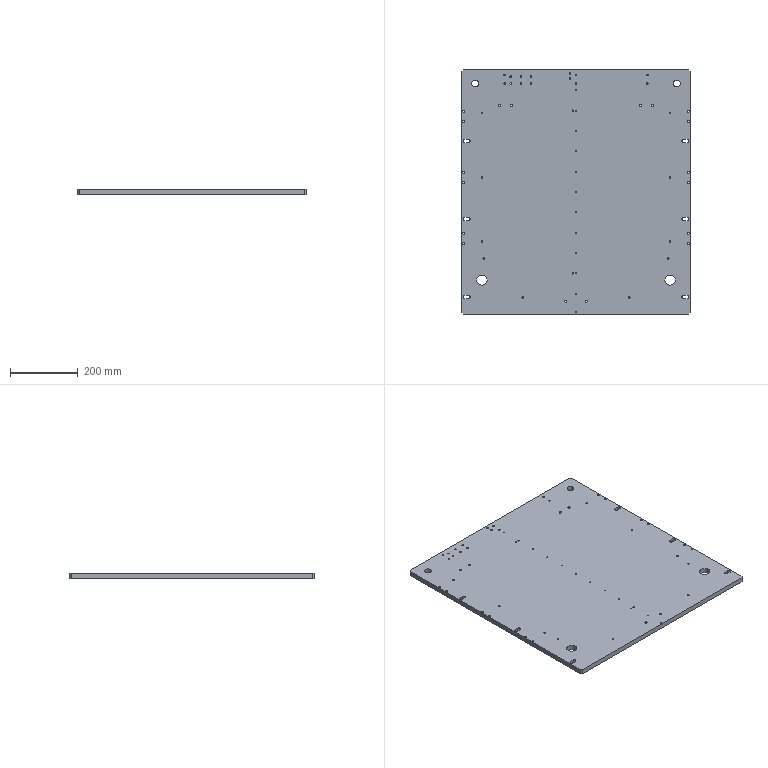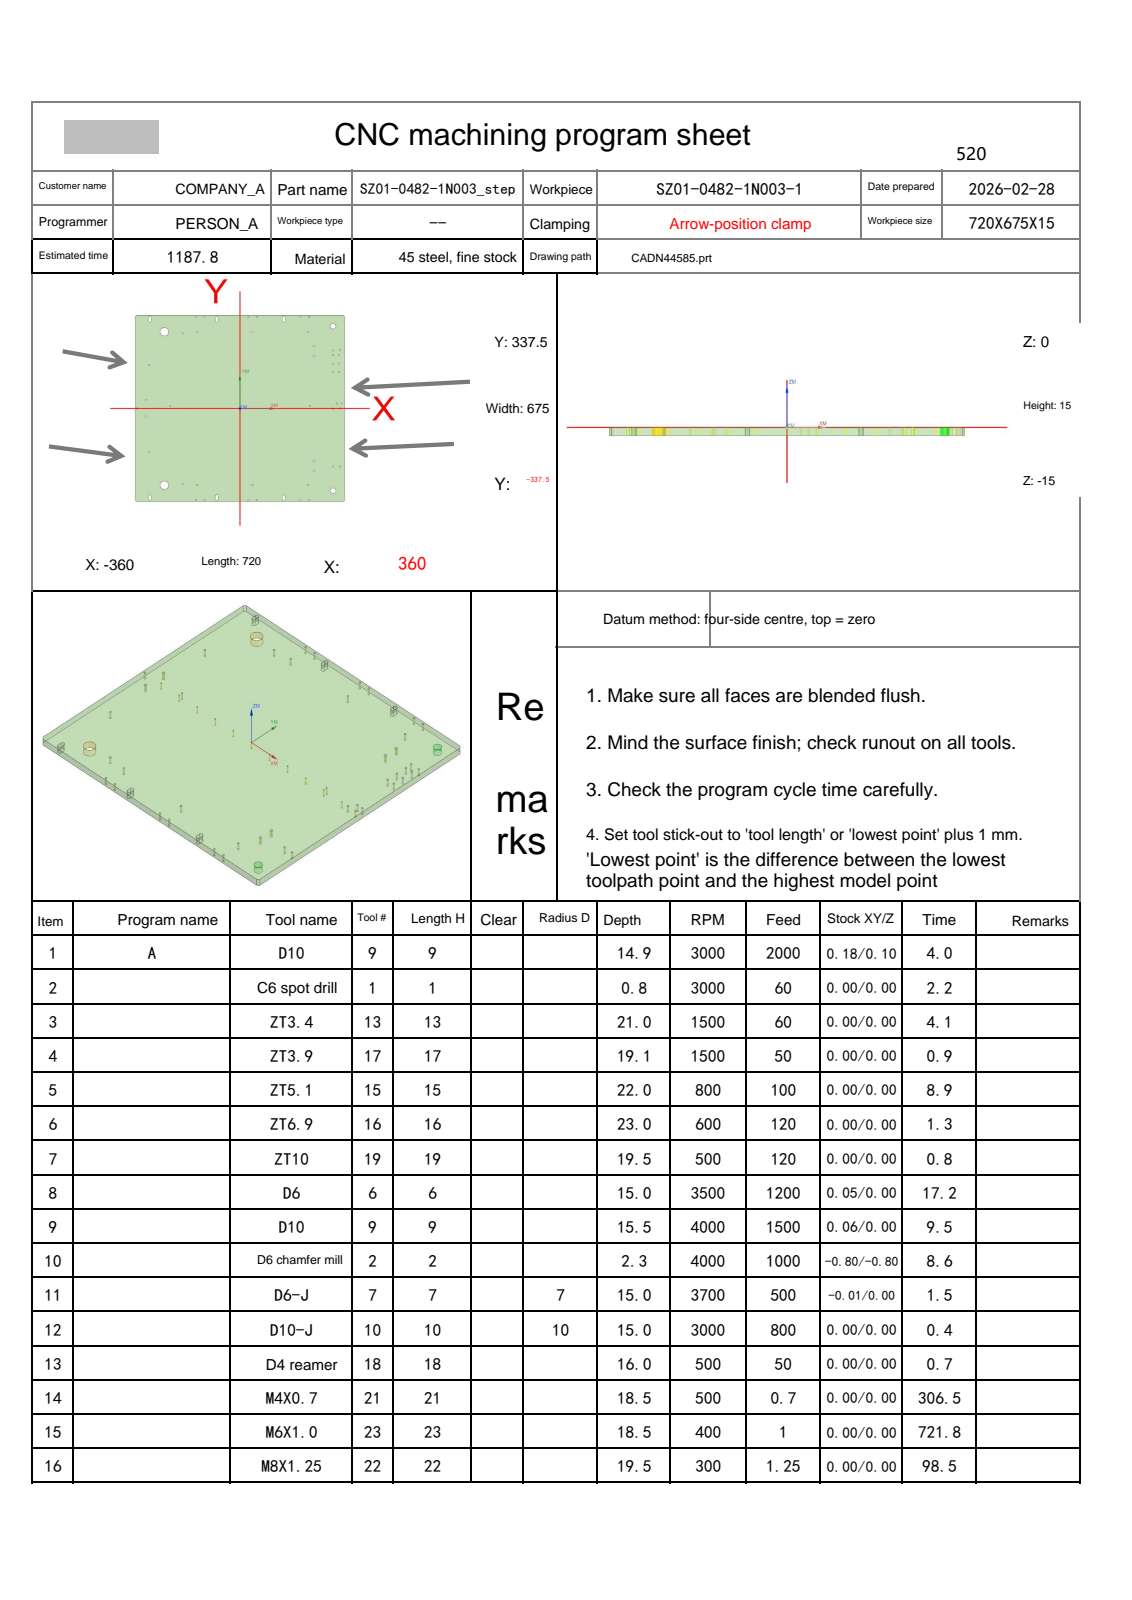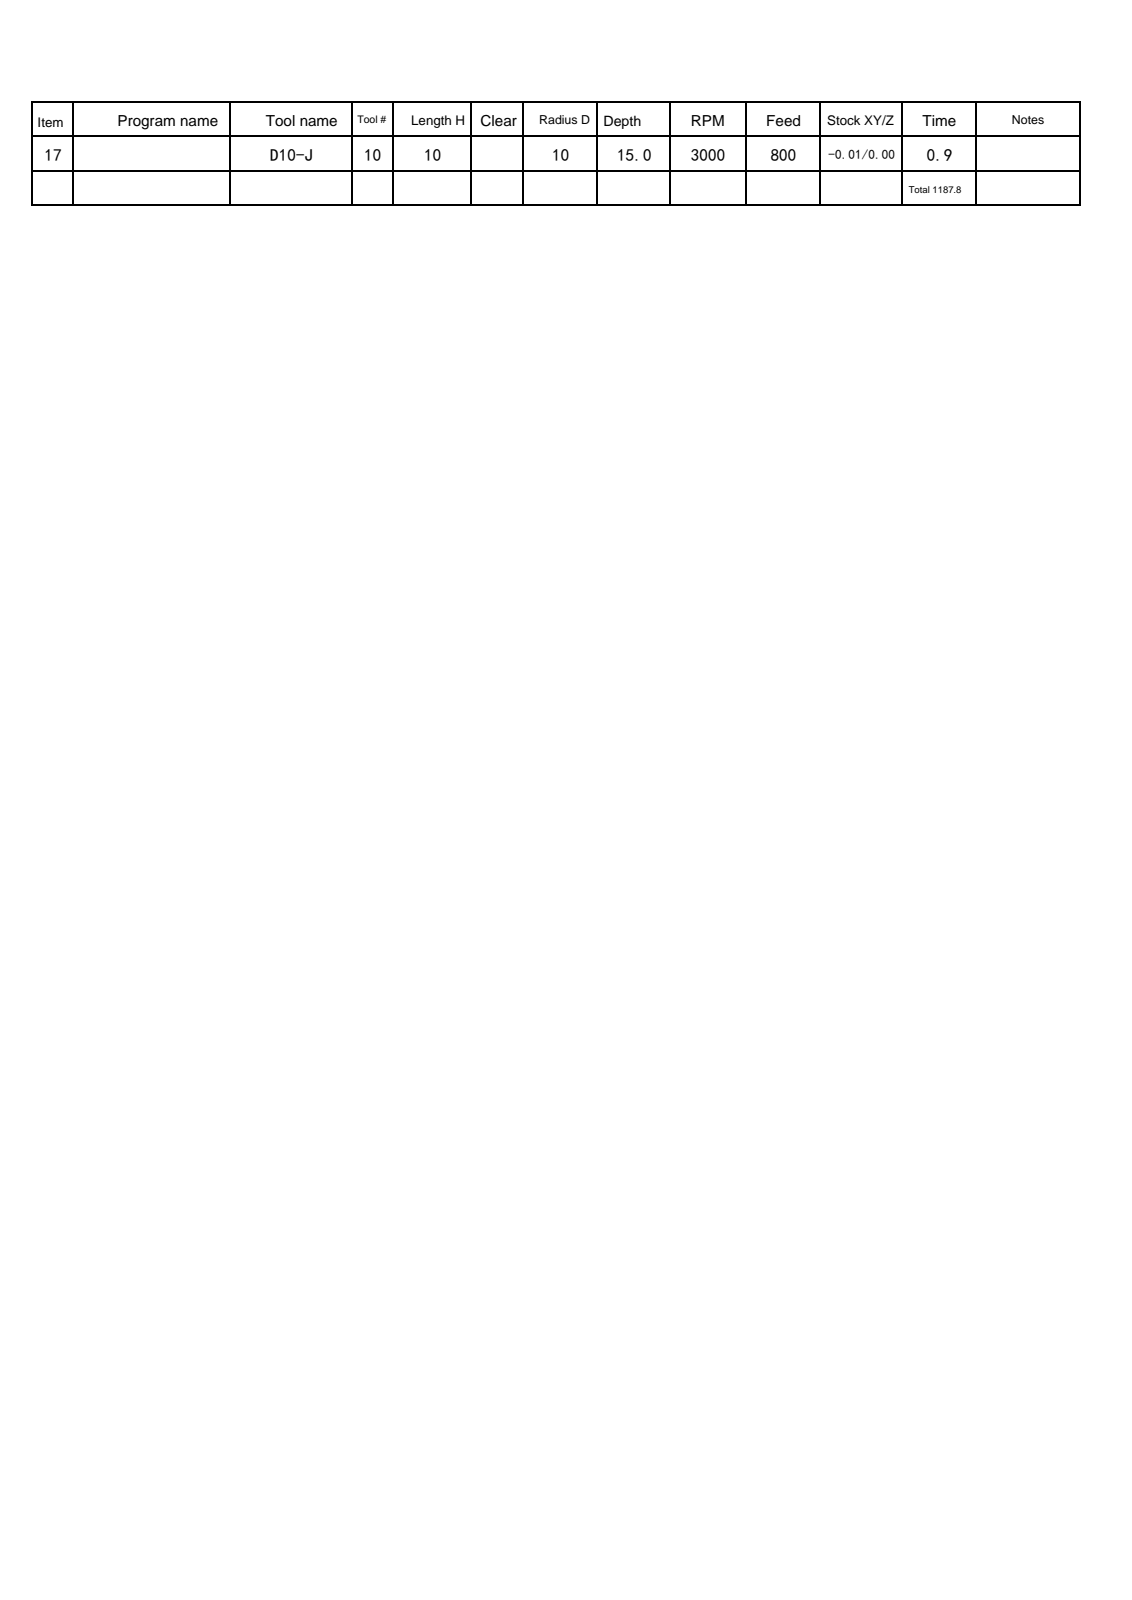NC program | NX | posted by the shop | part box 675 x 720 x 15 mm
Lines 7671 to 7907 of 7907:
N14 T21 M06
(M4X0.7 D=3.3 DR_a=180 H=21)
G00 G90 G54 X-300. Y0.0 M03 S500
G43 H21 Z30.
M08
G95
G98 G84 X-300. Y0.0 Z-18.5 R1. F.7 Q1.
X-240.
X-180.
X-120.
X-60.
X0.0
X60.
X120.
X180.
X240.
X300.
G80
G94
G00 Z30.
G91 G28 Z0.0
M05
M09
G91 G28 Z0.0
M01
N15 T23 M06
(M6X1.0 D=5. DR_a=180 H=23)
G00 G90 G54 X320. Y0.0 M03 S400
G43 H23 Z30.
M08
G95
G98 G84 X320. Y0.0 Z-18.5 R1. F1. Q2.
X345.
X350. Y18.
X334.
X340. Y132.5
X320.
Y162.5
X340.
Y192.5
X345. Y210.
X320. Y192.5
Y210.
X233. Y277.
X238. Y331.5
X208.
X58.
X28.
X43. Y277.
X-122. Y331.5
X-152.
X-147. Y277.
X-197. Y271.932
X-311.932 Y157.
X-354. Y0.0
X-311.932 Y-157.
X-197. Y-271.932
X-147. Y-277.
X-152. Y-331.5
X-122.
X43. Y-277.
X28. Y-331.5
X58.
X208.
X238.
X233. Y-277.
X320. Y-210.
X345.
G80
G94
G00 Z30.
G91 G28 Z0.0
M05
M09
G91 G28 Z0.0
M01
N16 T22 M06
(M8X1.25 D=6.8 DR_a=180 H=22)
G00 G90 G54 X255. Y225.5 M03 S300
G43 H22 Z30.
M08
G95
G98 G84 X255. Y225.5 Z-19.5 R1. F1.25 Q3.
Y189.5
Y-189.5
Y-225.5
X-322. Y-30.
Y30.
G80
G94
G00 Z30.
G91 G28 Z0.0
M05
M09
G91 G28 Z0.0
M01
N17 T10 M06
(D10-J  D=10. R=0. H=10 ce=-0.01 di=0.00)
G00 G90 G54 X322.973 Y296. M03 S3000
G43 H10 Z10.
M08
Z-6.
G01 Z-7.5 F600.
G41 D10
X323.51
G03 X325.01 Y297.5 I0.0 J1.5
X320. Y302.51 I-5.01 J0.0
X314.99 Y297.5 I0.0 J-5.01
X320. Y292.49 I5.01 J0.0
X325.01 Y297.5 I0.0 J5.01
X324.994 Y297.9 I-5.01 J0.0
X323.499 Y299.28 I-1.495 J-.12
G01 X323.379 Y299.275
X323.044 Y299.248
G40 X322.844 Y299.232
Z-6.
G00 X322.973 Y296.
Z-13.5
G01 Z-15.
G41 D10
X323.51
G03 X325.01 Y297.5 I0.0 J1.5
X320. Y302.51 I-5.01 J0.0
X314.99 Y297.5 I0.0 J-5.01
X320. Y292.49 I5.01 J0.0
X325.01 Y297.5 I0.0 J5.01
X324.994 Y297.9 I-5.01 J0.0
X323.499 Y299.28 I-1.495 J-.12
G01 X323.379 Y299.275
X323.044 Y299.248
G40 X322.844 Y299.232
Z-13.5
G00 Z10.
X322.973 Y-299.
Z-6.
G01 Z-7.5
G41 D10
X323.51
G03 X325.01 Y-297.5 I0.0 J1.5
X320. Y-292.49 I-5.01 J0.0
X314.99 Y-297.5 I0.0 J-5.01
X320. Y-302.51 I5.01 J0.0
X325.01 Y-297.5 I0.0 J5.01
X324.994 Y-297.1 I-5.01 J0.0
X323.499 Y-295.72 I-1.495 J-.12
G01 X323.379 Y-295.725
X323.044 Y-295.752
G40 X322.844 Y-295.768
Z-6.
G00 X322.973 Y-299.
Z-13.5
G01 Z-15.
G41 D10
X323.51
G03 X325.01 Y-297.5 I0.0 J1.5
X320. Y-292.49 I-5.01 J0.0
X314.99 Y-297.5 I0.0 J-5.01
X320. Y-302.51 I5.01 J0.0
X325.01 Y-297.5 I0.0 J5.01
X324.994 Y-297.1 I-5.01 J0.0
X323.499 Y-295.72 I-1.495 J-.12
G01 X323.379 Y-295.725
X323.044 Y-295.752
G40 X322.844 Y-295.768
Z-13.5
G00 Z10.
G00 G90 X354.293 Y345.278 M03 S3000
Z60.
Z-7.
G01 Z-8. F800.
X358.536 Y341.036
X363.536 Y336.036
X367.778 Y331.793
Z-7.
G00 Z60.
X354.293 Y345.278
Z-14.
G01 Z-15.
X358.536 Y341.036
X363.536 Y336.036
X367.778 Y331.793
Z-14.
G00 Z60.
Y-331.793
Z-7.
G01 Z-8.
X363.536 Y-336.036
X358.536 Y-341.036
X354.293 Y-345.278
Z-7.
G00 Z60.
X367.778 Y-331.793
Z-14.
G01 Z-15.
X363.536 Y-336.036
X358.536 Y-341.036
X354.293 Y-345.278
Z-14.
G00 Z60.
X-354.293
Z-7.
G01 Z-8.
X-358.536 Y-341.036
X-363.536 Y-336.036
X-367.778 Y-331.793
Z-7.
G00 Z60.
X-354.293 Y-345.278
Z-14.
G01 Z-15.
X-358.536 Y-341.036
X-363.536 Y-336.036
X-367.778 Y-331.793
Z-14.
G00 Z60.
Y331.793
Z-7.
G01 Z-8.
X-363.536 Y336.036
X-358.536 Y341.036
X-354.293 Y345.278
Z-7.
G00 Z60.
X-367.778 Y331.793
Z-14.
G01 Z-15.
X-363.536 Y336.036
X-358.536 Y341.036
X-354.293 Y345.278
Z-14.
G00 Z60.
M05
M09
G91 G28 Z0.0
G91 G28 Y0.0
M30
%